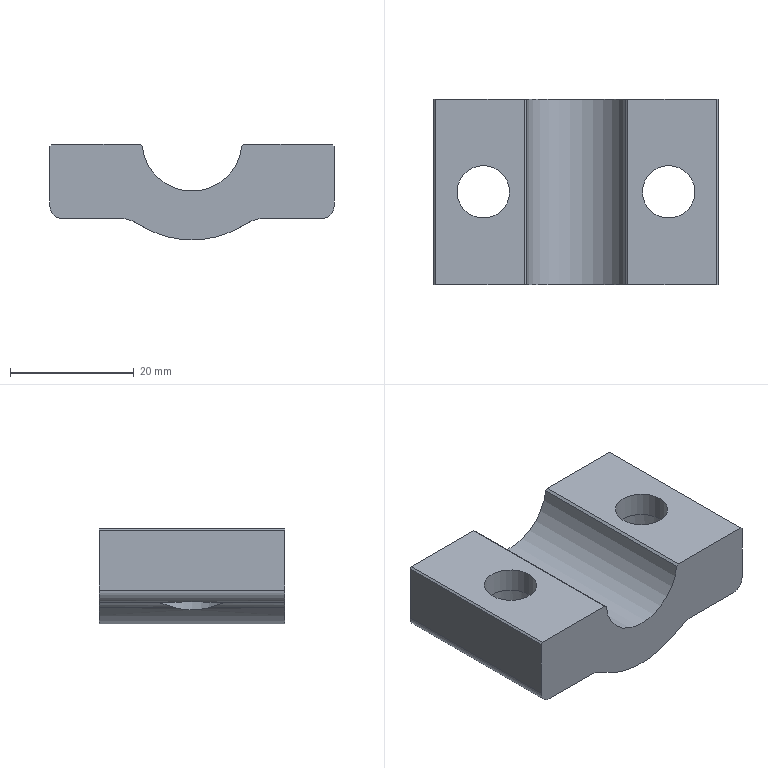CAM job | NX | 3+2 milling, drilling | part box 46 x 30 x 15.5 mm | stock box 50 x 34.5 x 20.5 mm
Tools:
number,name,description,diameter,corner_radius,flute_length,length,flutes
4,D10点钻,定心钻D10,10.0,0.0,87.0,133.0,2
2,D10开粗,D10,10.0,0.0,25.0,75.0,2
3,D10精光,D10,10.0,0.0,25.0,75.0,2
5,Z8.5,Z8.5直柄钻头,8.5,0.0,75.0,117.0,2
1,D50R6_1,圆形铣刀片,50.0,6.0,12.0,80.0,2
2,D10开粗_1,D10,10.0,0.0,40.0,75.0,2
Operations:
program,operation,operation_type,tool,method,geometry_group,spindle_rpm,surface_speed,feed_per_tooth,feed_cut,feed_plunge,cut_length_mm,path_length_mm,cut_time_min,machine_time_min
XX-CNC1,一刀光面,VolumeBased25DMillingOperation,D50R6_1,METHOD,MCS_1,2000.0,1187.0,0.1,800.0,100.0,112.041,166.041,0.1401,0.1455
XX-CNC1,ADAPTIVE_MILLING,CavityMilling,D10开粗_1,METHOD,W1,3000.0,100.0,0.1178,1500.0,100.0,3247.279,3363.279,1.651,1.662
XX-CNC1,PLANAR_MILL,PlanarMilling,D10精光,METHOD,W1,1061.0,100.0,0.1178,250.0,100.0,661.34,870.27,2.645,2.666
XX-CNC1,PLANAR_MILL_COPY,PlanarMilling,D10点钻,METHOD,W1,3000.0,100.0,0.1178,800.0,100.0,146.12,206.12,0.1827,0.1887
XX-CNC1,一刀光面_COPY_1,VolumeBased25DMillingOperation,D50R6_1,METHOD,MCS_1,2000.0,1187.0,0.1,800.0,100.0,112.041,166.041,0.1401,0.1455
XX-CNC2,一刀光面_COPY,VolumeBased25DMillingOperation,D50R6_1,METHOD,MCS_1,2000.0,1187.0,0.1,800.0,100.0,560.207,1233.772,0.7003,0.7676
XX-CNC2,一刀光面_COPY_COPY,VolumeBased25DMillingOperation,D50R6_1,METHOD,MCS_1,2000.0,1187.0,0.1,800.0,100.0,112.041,166.041,0.1401,0.1455
XX-CNC2,PLANAR_MILL_COPY_COPY,PlanarMilling,D10点钻,METHOD,W1,3000.0,100.0,0.1178,800.0,100.0,146.12,206.12,0.1827,0.1887
XX-CNC3,2D点孔,Operation,D10点钻,METHOD,MCS_3,2000.0,18.0,0.05,200.0,0.0,7.0,113.067,0.035,0.0456
XX-CNC3,2D点孔_COPY,Operation,Z8.5,METHOD,MCS_3,1600.0,18.0,0.05,150.0,0.0,34.0,167.067,0.2267,0.24
XX-CNC3,孔铣螺旋,CylinderMilling,D10开粗,METHOD,MCS_3,3000.0,188.0,0.1833,800.0,100.0,283.49,431.781,0.3544,0.3692
XX-CNC3,孔铣螺旋_COPY,CylinderMilling,D10精光,METHOD,MCS_3,3000.0,188.0,0.1833,300.0,100.0,32.987,201.696,0.11,0.1268